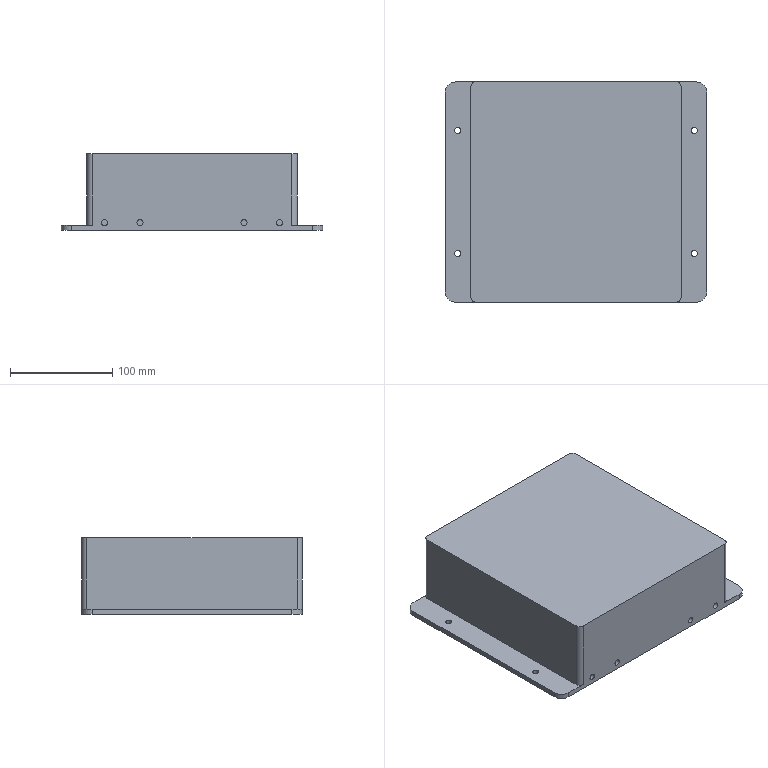NC program | NX | posted with a generic post | part box 255 x 215 x 75 mm
Lines 4678 to 5784 of 11258:
(ZLEVEL_PROFILE_COPY , TOOL : D10JING)
N9336 T14 M6
N9338 G54
N9340 G17 G0 G90 X87.615 Y-95.5 B0. C0. S9500 M3
N9342 G43 Z30. H14
N9344 Z0.5
N9346 G94 G1 Z-0.5 F1250.
N9348 X88.481 Y-97.
N9350 G3 X89.347 Y-97.5 R1.
N9352 G1 X92.492
N9354 X92.5 Y-97.459
N9356 Y-94.347
N9358 G3 X92. Y-93.481 R1.
N9360 G1 X90.5 Y-92.615
N9362 Z0.5
N9364 G0 X87.615 Y-95.5 Z0.
N9366 G1 Z-1.
N9368 X88.481 Y-97.
N9370 G3 X89.347 Y-97.5 R1.
N9372 G1 X92.492
N9374 X92.5 Y-97.459
N9376 Y-94.347
N9378 G3 X92. Y-93.481 R1.
N9380 G1 X90.5 Y-92.615
N9382 Z0.
N9384 G0 X87.615 Y-95.5 Z-0.5
N9386 G1 Z-1.5
N9388 X88.481 Y-97.
N9390 G3 X89.347 Y-97.5 R1.
N9392 G1 X92.492
N9394 X92.5 Y-97.459
N9396 Y-94.347
N9398 G3 X92. Y-93.481 R1.
N9400 G1 X90.5 Y-92.615
N9402 Z-0.5
N9404 G0 X87.615 Y-95.5 Z-1.
N9406 G1 Z-2.
N9408 X88.481 Y-97.
N9410 G3 X89.347 Y-97.5 R1.
N9412 G1 X92.492
N9414 X92.5 Y-97.459
N9416 Y-94.347
N9418 G3 X92. Y-93.481 R1.
N9420 G1 X90.5 Y-92.615
N9422 Z-1.
N9424 G0 X87.615 Y-95.5 Z-1.5
N9426 G1 Z-2.5
N9428 X88.481 Y-97.
N9430 G3 X89.347 Y-97.5 R1.
N9432 G1 X92.492
N9434 X92.5 Y-97.459
N9436 Y-94.347
N9438 G3 X92. Y-93.481 R1.
N9440 G1 X90.5 Y-92.615
N9442 Z-1.5
N9444 G0 X87.615 Y-95.5 Z-2.
N9446 G1 Z-3.
N9448 X88.481 Y-97.
N9450 G3 X89.347 Y-97.5 R1.
N9452 G1 X92.492
N9454 X92.5 Y-97.459
N9456 Y-94.347
N9458 G3 X92. Y-93.481 R1.
N9460 G1 X90.5 Y-92.615
N9462 Z-2.
N9464 G0 X87.615 Y-95.5 Z-2.5
N9466 G1 Z-3.5
N9468 X88.481 Y-97.
N9470 G3 X89.347 Y-97.5 R1.
N9472 G1 X92.492
N9474 X92.5 Y-97.459
N9476 Y-94.347
N9478 G3 X92. Y-93.481 R1.
N9480 G1 X90.5 Y-92.615
N9482 Z-2.5
N9484 G0 X87.615 Y-95.5 Z-3.
N9486 G1 Z-4.
N9488 X88.481 Y-97.
N9490 G3 X89.347 Y-97.5 R1.
N9492 G1 X92.492
N9494 X92.5 Y-97.459
N9496 Y-94.347
N9498 G3 X92. Y-93.481 R1.
N9500 G1 X90.5 Y-92.615
N9502 Z-3.
N9504 G0 X87.615 Y-95.5 Z-3.5
N9506 G1 Z-4.5
N9508 X88.481 Y-97.
N9510 G3 X89.347 Y-97.5 R1.
N9512 G1 X92.492
N9514 X92.5 Y-97.459
N9516 Y-94.347
N9518 G3 X92. Y-93.481 R1.
N9520 G1 X90.5 Y-92.615
N9522 Z-3.5
N9524 G0 X87.615 Y-95.5 Z-4.
N9526 G1 Z-5.
N9528 X88.481 Y-97.
N9530 G3 X89.347 Y-97.5 R1.
N9532 G1 X92.492
N9534 X92.5 Y-97.459
N9536 Y-94.347
N9538 G3 X92. Y-93.481 R1.
N9540 G1 X90.5 Y-92.615
N9542 Z-4.
N9544 G0 X87.615 Y-95.5 Z-4.5
N9546 G1 Z-5.5
N9548 X88.481 Y-97.
N9550 G3 X89.347 Y-97.5 R1.
N9552 G1 X92.492
N9554 X92.5 Y-97.459
N9556 Y-94.347
N9558 G3 X92. Y-93.481 R1.
N9560 G1 X90.5 Y-92.615
N9562 Z-4.5
N9564 G0 X87.615 Y-95.5 Z-5.
N9566 G1 Z-6.
N9568 X88.481 Y-97.
N9570 G3 X89.347 Y-97.5 R1.
N9572 G1 X92.492
N9574 X92.5 Y-97.459
N9576 Y-94.347
N9578 G3 X92. Y-93.481 R1.
N9580 G1 X90.5 Y-92.615
N9582 Z-5.
N9584 G0 X87.615 Y-95.5 Z-5.5
N9586 G1 Z-6.5
N9588 X88.481 Y-97.
N9590 G3 X89.347 Y-97.5 R1.
N9592 G1 X92.492
N9594 X92.5 Y-97.459
N9596 Y-94.347
N9598 G3 X92. Y-93.481 R1.
N9600 G1 X90.5 Y-92.615
N9602 Z-5.5
N9604 G0 X87.615 Y-95.5 Z-6.
N9606 G1 Z-7.
N9608 X88.481 Y-97.
N9610 G3 X89.347 Y-97.5 R1.
N9612 G1 X92.492
N9614 X92.5 Y-97.459
N9616 Y-94.347
N9618 G3 X92. Y-93.481 R1.
N9620 G1 X90.5 Y-92.615
N9622 Z-6.
N9624 G0 X87.615 Y-95.5 Z-6.5
N9626 G1 Z-7.5
N9628 X88.481 Y-97.
N9630 G3 X89.347 Y-97.5 R1.
N9632 G1 X92.492
N9634 X92.5 Y-97.459
N9636 Y-94.347
N9638 G3 X92. Y-93.481 R1.
N9640 G1 X90.5 Y-92.615
N9642 Z-6.5
N9644 G0 X87.615 Y-95.5 Z-7.
N9646 G1 Z-8.
N9648 X88.481 Y-97.
N9650 G3 X89.347 Y-97.5 R1.
N9652 G1 X92.492
N9654 X92.5 Y-97.459
N9656 Y-94.347
N9658 G3 X92. Y-93.481 R1.
N9660 G1 X90.5 Y-92.615
N9662 Z-7.
N9664 G0 X87.615 Y-95.5 Z-7.5
N9666 G1 Z-8.5
N9668 X88.481 Y-97.
N9670 G3 X89.347 Y-97.5 R1.
N9672 G1 X92.492
N9674 X92.5 Y-97.459
N9676 Y-94.347
N9678 G3 X92. Y-93.481 R1.
N9680 G1 X90.5 Y-92.615
N9682 Z-7.5
N9684 G0 X87.615 Y-95.5 Z-8.
N9686 G1 Z-9.
N9688 X88.481 Y-97.
N9690 G3 X89.347 Y-97.5 R1.
N9692 G1 X92.492
N9694 X92.5 Y-97.459
N9696 Y-94.347
N9698 G3 X92. Y-93.481 R1.
N9700 G1 X90.5 Y-92.615
N9702 Z-8.
N9704 G0 X87.615 Y-95.5 Z-8.5
N9706 G1 Z-9.5
N9708 X88.481 Y-97.
N9710 G3 X89.347 Y-97.5 R1.
N9712 G1 X92.492
N9714 X92.5 Y-97.459
N9716 Y-94.347
N9718 G3 X92. Y-93.481 R1.
N9720 G1 X90.5 Y-92.615
N9722 Z-8.5
N9724 G0 X87.615 Y-95.5 Z-9.
N9726 G1 Z-10.
N9728 X88.481 Y-97.
N9730 G3 X89.347 Y-97.5 R1.
N9732 G1 X92.492
N9734 X92.5 Y-97.459
N9736 Y-94.347
N9738 G3 X92. Y-93.481 R1.
N9740 G1 X90.5 Y-92.615
N9742 Z-9.
N9744 G0 X87.615 Y-95.5 Z-9.5
N9746 G1 Z-10.5
N9748 X88.481 Y-97.
N9750 G3 X89.347 Y-97.5 R1.
N9752 G1 X92.492
N9754 X92.5 Y-97.459
N9756 Y-94.347
N9758 G3 X92. Y-93.481 R1.
N9760 G1 X90.5 Y-92.615
N9762 Z-9.5
N9764 G0 X87.615 Y-95.5 Z-10.
N9766 G1 Z-11.
N9768 X88.481 Y-97.
N9770 G3 X89.347 Y-97.5 R1.
N9772 G1 X92.492
N9774 X92.5 Y-97.459
N9776 Y-94.347
N9778 G3 X92. Y-93.481 R1.
N9780 G1 X90.5 Y-92.615
N9782 Z-10.
N9784 G0 X87.615 Y-95.5 Z-10.5
N9786 G1 Z-11.5
N9788 X88.481 Y-97.
N9790 G3 X89.347 Y-97.5 R1.
N9792 G1 X92.492
N9794 X92.5 Y-97.459
N9796 Y-94.347
N9798 G3 X92. Y-93.481 R1.
N9800 G1 X90.5 Y-92.615
N9802 Z-10.5
N9804 G0 X87.615 Y-95.5 Z-11.
N9806 G1 Z-12.
N9808 X88.481 Y-97.
N9810 G3 X89.347 Y-97.5 R1.
N9812 G1 X92.492
N9814 X92.5 Y-97.459
N9816 Y-94.347
N9818 G3 X92. Y-93.481 R1.
N9820 G1 X90.5 Y-92.615
N9822 Z-11.
N9824 G0 X87.615 Y-95.5 Z-11.5
N9826 G1 Z-12.5
N9828 X88.481 Y-97.
N9830 G3 X89.347 Y-97.5 R1.
N9832 G1 X92.492
N9834 X92.5 Y-97.459
N9836 Y-94.347
N9838 G3 X92. Y-93.481 R1.
N9840 G1 X90.5 Y-92.615
N9842 Z-11.5
N9844 G0 X87.615 Y-95.5 Z-12.
N9846 G1 Z-13.
N9848 X88.481 Y-97.
N9850 G3 X89.347 Y-97.5 R1.
N9852 G1 X92.492
N9854 X92.5 Y-97.459
N9856 Y-94.347
N9858 G3 X92. Y-93.481 R1.
N9860 G1 X90.5 Y-92.615
N9862 Z-12.
N9864 G0 X87.615 Y-95.5 Z-12.5
N9866 G1 Z-13.5
N9868 X88.481 Y-97.
N9870 G3 X89.347 Y-97.5 R1.
N9872 G1 X92.492
N9874 X92.5 Y-97.459
N9876 Y-94.347
N9878 G3 X92. Y-93.481 R1.
N9880 G1 X90.5 Y-92.615
N9882 Z-12.5
N9884 G0 X87.615 Y-95.5 Z-13.
N9886 G1 Z-14.
N9888 X88.481 Y-97.
N9890 G3 X89.347 Y-97.5 R1.
N9892 G1 X92.492
N9894 X92.5 Y-97.459
N9896 Y-94.347
N9898 G3 X92. Y-93.481 R1.
N9900 G1 X90.5 Y-92.615
N9902 Z-13.
N9904 G0 X87.615 Y-95.5 Z-13.5
N9906 G1 Z-14.5
N9908 X88.481 Y-97.
N9910 G3 X89.347 Y-97.5 R1.
N9912 G1 X92.492
N9914 X92.5 Y-97.459
N9916 Y-94.347
N9918 G3 X92. Y-93.481 R1.
N9920 G1 X90.5 Y-92.615
N9922 Z-13.5
N9924 G0 X87.615 Y-95.5 Z-14.
N9926 G1 Z-15.
N9928 X88.481 Y-97.
N9930 G3 X89.347 Y-97.5 R1.
N9932 G1 X92.492
N9934 X92.5 Y-97.459
N9936 Y-94.347
N9938 G3 X92. Y-93.481 R1.
N9940 G1 X90.5 Y-92.615
N9942 Z-14.
N9944 G0 X87.615 Y-95.5 Z-14.5
N9946 G1 Z-15.5
N9948 X88.481 Y-97.
N9950 G3 X89.347 Y-97.5 R1.
N9952 G1 X92.492
N9954 X92.5 Y-97.459
N9956 Y-94.347
N9958 G3 X92. Y-93.481 R1.
N9960 G1 X90.5 Y-92.615
N9962 Z-14.5
N9964 G0 X87.615 Y-95.5 Z-15.
N9966 G1 Z-16.
N9968 X88.481 Y-97.
N9970 G3 X89.347 Y-97.5 R1.
N9972 G1 X92.492
N9974 X92.5 Y-97.459
N9976 Y-94.347
N9978 G3 X92. Y-93.481 R1.
N9980 G1 X90.5 Y-92.615
N9982 Z-15.
N9984 G0 X87.615 Y-95.5 Z-15.5
N9986 G1 Z-16.5
N9988 X88.481 Y-97.
N9990 G3 X89.347 Y-97.5 R1.
N9992 G1 X92.492
N9994 X92.5 Y-97.459
N9996 Y-94.347
N9998 G3 X92. Y-93.481 R1.
N10000 G1 X90.5 Y-92.615
N10002 Z-15.5
N10004 G0 X87.615 Y-95.5 Z-16.
N10006 G1 Z-17.
N10008 X88.481 Y-97.
N10010 G3 X89.347 Y-97.5 R1.
N10012 G1 X92.492
N10014 X92.5 Y-97.459
N10016 Y-94.347
N10018 G3 X92. Y-93.481 R1.
N10020 G1 X90.5 Y-92.615
N10022 Z-16.
N10024 G0 X87.615 Y-95.5 Z-16.5
N10026 G1 Z-17.5
N10028 X88.481 Y-97.
N10030 G3 X89.347 Y-97.5 R1.
N10032 G1 X92.492
N10034 X92.5 Y-97.459
N10036 Y-94.347
N10038 G3 X92. Y-93.481 R1.
N10040 G1 X90.5 Y-92.615
N10042 Z-16.5
N10044 G0 X87.615 Y-95.5 Z-17.
N10046 G1 Z-18.
N10048 X88.481 Y-97.
N10050 G3 X89.347 Y-97.5 R1.
N10052 G1 X92.492
N10054 X92.5 Y-97.459
N10056 Y-94.347
N10058 G3 X92. Y-93.481 R1.
N10060 G1 X90.5 Y-92.615
N10062 Z-17.
N10064 G0 X87.615 Y-95.5 Z-17.5
N10066 G1 Z-18.5
N10068 X88.481 Y-97.
N10070 G3 X89.347 Y-97.5 R1.
N10072 G1 X92.492
N10074 X92.5 Y-97.459
N10076 Y-94.347
N10078 G3 X92. Y-93.481 R1.
N10080 G1 X90.5 Y-92.615
N10082 Z-17.5
N10084 G0 X87.615 Y-95.5 Z-18.
N10086 G1 Z-19.
N10088 X88.481 Y-97.
N10090 G3 X89.347 Y-97.5 R1.
N10092 G1 X92.492
N10094 X92.5 Y-97.459
N10096 Y-94.347
N10098 G3 X92. Y-93.481 R1.
N10100 G1 X90.5 Y-92.615
N10102 Z-18.
N10104 G0 X87.615 Y-95.5 Z-18.5
N10106 G1 Z-19.5
N10108 X88.481 Y-97.
N10110 G3 X89.347 Y-97.5 R1.
N10112 G1 X92.492
N10114 X92.5 Y-97.459
N10116 Y-94.347
N10118 G3 X92. Y-93.481 R1.
N10120 G1 X90.5 Y-92.615
N10122 Z-18.5
N10124 G0 X87.615 Y-95.5 Z-19.
N10126 G1 Z-20.
N10128 X88.481 Y-97.
N10130 G3 X89.347 Y-97.5 R1.
N10132 G1 X92.492
N10134 X92.5 Y-97.459
N10136 Y-94.347
N10138 G3 X92. Y-93.481 R1.
N10140 G1 X90.5 Y-92.615
N10142 Z-19.
N10144 G0 X87.615 Y-95.5 Z-19.5
N10146 G1 Z-20.5
N10148 X88.481 Y-97.
N10150 G3 X89.347 Y-97.5 R1.
N10152 G1 X92.492
N10154 X92.5 Y-97.459
N10156 Y-94.347
N10158 G3 X92. Y-93.481 R1.
N10160 G1 X90.5 Y-92.615
N10162 Z-19.5
N10164 G0 X87.615 Y-95.5 Z-20.
N10166 G1 Z-21.
N10168 X88.481 Y-97.
N10170 G3 X89.347 Y-97.5 R1.
N10172 G1 X92.492
N10174 X92.5 Y-97.459
N10176 Y-94.347
N10178 G3 X92. Y-93.481 R1.
N10180 G1 X90.5 Y-92.615
N10182 Z-20.
N10184 G0 X87.615 Y-95.5 Z-20.5
N10186 G1 Z-21.5
N10188 X88.481 Y-97.
N10190 G3 X89.347 Y-97.5 R1.
N10192 G1 X92.492
N10194 X92.5 Y-97.459
N10196 Y-94.347
N10198 G3 X92. Y-93.481 R1.
N10200 G1 X90.5 Y-92.615
N10202 Z-20.5
N10204 G0 X87.615 Y-95.5 Z-21.
N10206 G1 Z-22.
N10208 X88.481 Y-97.
N10210 G3 X89.347 Y-97.5 R1.
N10212 G1 X92.492
N10214 X92.5 Y-97.459
N10216 Y-94.347
N10218 G3 X92. Y-93.481 R1.
N10220 G1 X90.5 Y-92.615
N10222 Z-21.
N10224 G0 X87.615 Y-95.5 Z-21.5
N10226 G1 Z-22.5
N10228 X88.481 Y-97.
N10230 G3 X89.347 Y-97.5 R1.
N10232 G1 X92.492
N10234 X92.5 Y-97.459
N10236 Y-94.347
N10238 G3 X92. Y-93.481 R1.
N10240 G1 X90.5 Y-92.615
N10242 Z-21.5
N10244 G0 X87.615 Y-95.5 Z-22.
N10246 G1 Z-23.
N10248 X88.481 Y-97.
N10250 G3 X89.347 Y-97.5 R1.
N10252 G1 X92.492
N10254 X92.5 Y-97.459
N10256 Y-94.347
N10258 G3 X92. Y-93.481 R1.
N10260 G1 X90.5 Y-92.615
N10262 Z-22.
N10264 G0 X87.615 Y-95.5 Z-22.5
N10266 G1 Z-23.5
N10268 X88.481 Y-97.
N10270 G3 X89.347 Y-97.5 R1.
N10272 G1 X92.492
N10274 X92.5 Y-97.459
N10276 Y-94.347
N10278 G3 X92. Y-93.481 R1.
N10280 G1 X90.5 Y-92.615
N10282 Z-22.5
N10284 G0 X87.615 Y-95.5 Z-23.
N10286 G1 Z-24.
N10288 X88.481 Y-97.
N10290 G3 X89.347 Y-97.5 R1.
N10292 G1 X92.492
N10294 X92.5 Y-97.459
N10296 Y-94.347
N10298 G3 X92. Y-93.481 R1.
N10300 G1 X90.5 Y-92.615
N10302 Z-23.
N10304 G0 X87.615 Y-95.5 Z-23.5
N10306 G1 Z-24.5
N10308 X88.481 Y-97.
N10310 G3 X89.347 Y-97.5 R1.
N10312 G1 X92.492
N10314 X92.5 Y-97.459
N10316 Y-94.347
N10318 G3 X92. Y-93.481 R1.
N10320 G1 X90.5 Y-92.615
N10322 Z-23.5
N10324 G0 X87.615 Y-95.5 Z-24.
N10326 G1 Z-25.
N10328 X88.481 Y-97.
N10330 G3 X89.347 Y-97.5 R1.
N10332 G1 X92.492
N10334 X92.5 Y-97.459
N10336 Y-94.347
N10338 G3 X92. Y-93.481 R1.
N10340 G1 X90.5 Y-92.615
N10342 Z-24.
N10344 G0 X87.615 Y-95.5 Z-24.5
N10346 G1 Z-25.5
N10348 X88.481 Y-97.
N10350 G3 X89.347 Y-97.5 R1.
N10352 G1 X92.492
N10354 X92.5 Y-97.459
N10356 Y-94.347
N10358 G3 X92. Y-93.481 R1.
N10360 G1 X90.5 Y-92.615
N10362 Z-24.5
N10364 G0 X87.615 Y-95.5 Z-25.
N10366 G1 Z-26.
N10368 X88.481 Y-97.
N10370 G3 X89.347 Y-97.5 R1.
N10372 G1 X92.492
N10374 X92.5 Y-97.459
N10376 Y-94.347
N10378 G3 X92. Y-93.481 R1.
N10380 G1 X90.5 Y-92.615
N10382 Z-25.
N10384 G0 X87.615 Y-95.5 Z-25.5
N10386 G1 Z-26.5
N10388 X88.481 Y-97.
N10390 G3 X89.347 Y-97.5 R1.
N10392 G1 X92.492
N10394 X92.5 Y-97.459
N10396 Y-94.347
N10398 G3 X92. Y-93.481 R1.
N10400 G1 X90.5 Y-92.615
N10402 Z-25.5
N10404 G0 X87.615 Y-95.5 Z-26.
N10406 G1 Z-27.
N10408 X88.481 Y-97.
N10410 G3 X89.347 Y-97.5 R1.
N10412 G1 X92.492
N10414 X92.5 Y-97.459
N10416 Y-94.347
N10418 G3 X92. Y-93.481 R1.
N10420 G1 X90.5 Y-92.615
N10422 Z-26.
N10424 G0 X87.615 Y-95.5 Z-26.5
N10426 G1 Z-27.5
N10428 X88.481 Y-97.
N10430 G3 X89.347 Y-97.5 R1.
N10432 G1 X92.492
N10434 X92.5 Y-97.459
N10436 Y-94.347
N10438 G3 X92. Y-93.481 R1.
N10440 G1 X90.5 Y-92.615
N10442 Z-26.5
N10444 G0 X87.615 Y-95.5 Z-27.
N10446 G1 Z-28.
N10448 X88.481 Y-97.
N10450 G3 X89.347 Y-97.5 R1.
N10452 G1 X92.492
N10454 X92.5 Y-97.459
N10456 Y-94.347
N10458 G3 X92. Y-93.481 R1.
N10460 G1 X90.5 Y-92.615
N10462 Z-27.
N10464 G0 X87.615 Y-95.5 Z-27.5
N10466 G1 Z-28.5
N10468 X88.481 Y-97.
N10470 G3 X89.347 Y-97.5 R1.
N10472 G1 X92.492
N10474 X92.5 Y-97.459
N10476 Y-94.347
N10478 G3 X92. Y-93.481 R1.
N10480 G1 X90.5 Y-92.615
N10482 Z-27.5
N10484 G0 X87.615 Y-95.5 Z-28.
N10486 G1 Z-29.
N10488 X88.481 Y-97.
N10490 G3 X89.347 Y-97.5 R1.
N10492 G1 X92.492
N10494 X92.5 Y-97.459
N10496 Y-94.347
N10498 G3 X92. Y-93.481 R1.
N10500 G1 X90.5 Y-92.615
N10502 Z-28.
N10504 G0 X87.615 Y-95.5 Z-28.5
N10506 G1 Z-29.5
N10508 X88.481 Y-97.
N10510 G3 X89.347 Y-97.5 R1.
N10512 G1 X92.492
N10514 X92.5 Y-97.459
N10516 Y-94.347
N10518 G3 X92. Y-93.481 R1.
N10520 G1 X90.5 Y-92.615
N10522 Z-28.5
N10524 G0 X87.615 Y-95.5 Z-29.
N10526 G1 Z-30.
N10528 X88.481 Y-97.
N10530 G3 X89.347 Y-97.5 R1.
N10532 G1 X92.492
N10534 X92.5 Y-97.459
N10536 Y-94.347
N10538 G3 X92. Y-93.481 R1.
N10540 G1 X90.5 Y-92.615
N10542 Z-29.
N10544 G0 X87.615 Y-95.5 Z-29.5
N10546 G1 Z-30.5
N10548 X88.481 Y-97.
N10550 G3 X89.347 Y-97.5 R1.
N10552 G1 X92.492
N10554 X92.5 Y-97.459
N10556 Y-94.347
N10558 G3 X92. Y-93.481 R1.
N10560 G1 X90.5 Y-92.615
N10562 Z-29.5
N10564 G0 X87.615 Y-95.5 Z-30.
N10566 G1 Z-31.
N10568 X88.481 Y-97.
N10570 G3 X89.347 Y-97.5 R1.
N10572 G1 X92.492
N10574 X92.5 Y-97.459
N10576 Y-94.347
N10578 G3 X92. Y-93.481 R1.
N10580 G1 X90.5 Y-92.615
N10582 Z-30.
N10584 G0 X87.615 Y-95.5 Z-30.5
N10586 G1 Z-31.5
N10588 X88.481 Y-97.
N10590 G3 X89.347 Y-97.5 R1.
N10592 G1 X92.492
N10594 X92.5 Y-97.459
N10596 Y-94.347
N10598 G3 X92. Y-93.481 R1.
N10600 G1 X90.5 Y-92.615
N10602 Z-30.5
N10604 G0 X87.615 Y-95.5 Z-31.
N10606 G1 Z-32.
N10608 X88.481 Y-97.
N10610 G3 X89.347 Y-97.5 R1.
N10612 G1 X92.492
N10614 X92.5 Y-97.459
N10616 Y-94.347
N10618 G3 X92. Y-93.481 R1.
N10620 G1 X90.5 Y-92.615
N10622 Z-31.
N10624 G0 X87.615 Y-95.5 Z-31.5
N10626 G1 Z-32.5
N10628 X88.481 Y-97.
N10630 G3 X89.347 Y-97.5 R1.
N10632 G1 X92.492
N10634 X92.5 Y-97.459
N10636 Y-94.347
N10638 G3 X92. Y-93.481 R1.
N10640 G1 X90.5 Y-92.615
N10642 Z-31.5
N10644 G0 X87.615 Y-95.5 Z-32.
N10646 G1 Z-33.
N10648 X88.481 Y-97.
N10650 G3 X89.347 Y-97.5 R1.
N10652 G1 X92.492
N10654 X92.5 Y-97.459
N10656 Y-94.347
N10658 G3 X92. Y-93.481 R1.
N10660 G1 X90.5 Y-92.615
N10662 Z-32.
N10664 G0 X87.615 Y-95.5 Z-32.5
N10666 G1 Z-33.5
N10668 X88.481 Y-97.
N10670 G3 X89.347 Y-97.5 R1.
N10672 G1 X92.492
N10674 X92.5 Y-97.459
N10676 Y-94.347
N10678 G3 X92. Y-93.481 R1.
N10680 G1 X90.5 Y-92.615
N10682 Z-32.5
N10684 G0 X87.615 Y-95.5 Z-33.
N10686 G1 Z-34.
N10688 X88.481 Y-97.
N10690 G3 X89.347 Y-97.5 R1.
N10692 G1 X92.492
N10694 X92.5 Y-97.459
N10696 Y-94.347
N10698 G3 X92. Y-93.481 R1.
N10700 G1 X90.5 Y-92.615
N10702 Z-33.
N10704 G0 X87.615 Y-95.5 Z-33.5
N10706 G1 Z-34.5
N10708 X88.481 Y-97.
N10710 G3 X89.347 Y-97.5 R1.
N10712 G1 X92.492
N10714 X92.5 Y-97.459
N10716 Y-94.347
N10718 G3 X92. Y-93.481 R1.
N10720 G1 X90.5 Y-92.615
N10722 Z-33.5
N10724 G0 X87.615 Y-95.5 Z-34.
N10726 G1 Z-35.
N10728 X88.481 Y-97.
N10730 G3 X89.347 Y-97.5 R1.
N10732 G1 X92.492
N10734 X92.5 Y-97.459
N10736 Y-94.347
N10738 G3 X92. Y-93.481 R1.
N10740 G1 X90.5 Y-92.615
N10742 Z-34.
N10744 G0 X87.615 Y-95.5 Z-34.5
N10746 G1 Z-35.5
N10748 X88.481 Y-97.
N10750 G3 X89.347 Y-97.5 R1.
N10752 G1 X92.492
N10754 X92.5 Y-97.459
N10756 Y-94.347
N10758 G3 X92. Y-93.481 R1.
N10760 G1 X90.5 Y-92.615
N10762 Z-34.5
N10764 G0 X87.615 Y-95.5 Z-35.
N10766 G1 Z-36.
N10768 X88.481 Y-97.
N10770 G3 X89.347 Y-97.5 R1.
N10772 G1 X92.492
N10774 X92.5 Y-97.459
N10776 Y-94.347
N10778 G3 X92. Y-93.481 R1.
N10780 G1 X90.5 Y-92.615
N10782 Z-35.
N10784 G0 X87.615 Y-95.5 Z-35.5
N10786 G1 Z-36.5
N10788 X88.481 Y-97.
N10790 G3 X89.347 Y-97.5 R1.
N10792 G1 X92.492
N10794 X92.5 Y-97.459
N10796 Y-94.347
N10798 G3 X92. Y-93.481 R1.
N10800 G1 X90.5 Y-92.615
N10802 Z-35.5
N10804 G0 X87.615 Y-95.5 Z-36.
N10806 G1 Z-37.
N10808 X88.481 Y-97.
N10810 G3 X89.347 Y-97.5 R1.
N10812 G1 X92.492
N10814 X92.5 Y-97.459
N10816 Y-94.347
N10818 G3 X92. Y-93.481 R1.
N10820 G1 X90.5 Y-92.615
N10822 Z-36.
N10824 G0 X87.615 Y-95.5 Z-36.5
N10826 G1 Z-37.5
N10828 X88.481 Y-97.
N10830 G3 X89.347 Y-97.5 R1.
N10832 G1 X92.492
N10834 X92.5 Y-97.459
N10836 Y-94.347
N10838 G3 X92. Y-93.481 R1.
N10840 G1 X90.5 Y-92.615
N10842 Z-36.5
N10844 G0 X87.615 Y-95.5 Z-37.
N10846 G1 Z-38.
N10848 X88.481 Y-97.
N10850 G3 X89.347 Y-97.5 R1.
N10852 G1 X92.492
N10854 X92.5 Y-97.459
N10856 Y-94.347
N10858 G3 X92. Y-93.481 R1.
N10860 G1 X90.5 Y-92.615
N10862 Z-37.
N10864 G0 X87.615 Y-95.5 Z-37.5
N10866 G1 Z-38.5
N10868 X88.481 Y-97.
N10870 G3 X89.347 Y-97.5 R1.
N10872 G1 X92.492
N10874 X92.5 Y-97.459
N10876 Y-94.347
N10878 G3 X92. Y-93.481 R1.
N10880 G1 X90.5 Y-92.615
N10882 Z-37.5
N10884 G0 X87.615 Y-95.5 Z-38.
N10886 G1 Z-39.
N10888 X88.481 Y-97.
N10890 G3 X89.347 Y-97.5 R1.
N10892 G1 X92.492
N10894 X92.5 Y-97.459
N10896 Y-94.347
N10898 G3 X92. Y-93.481 R1.
N10900 G1 X90.5 Y-92.615
N10902 Z-38.
N10904 G0 X87.615 Y-95.5 Z-38.5
N10906 G1 Z-39.5
N10908 X88.481 Y-97.
N10910 G3 X89.347 Y-97.5 R1.
N10912 G1 X92.492
N10914 X92.5 Y-97.459
N10916 Y-94.347
N10918 G3 X92. Y-93.481 R1.
N10920 G1 X90.5 Y-92.615
N10922 Z-38.5
N10924 G0 X87.615 Y-95.5 Z-39.
N10926 G1 Z-40.
N10928 X88.481 Y-97.
N10930 G3 X89.347 Y-97.5 R1.
N10932 G1 X92.492
N10934 X92.5 Y-97.459
N10936 Y-94.347
N10938 G3 X92. Y-93.481 R1.
N10940 G1 X90.5 Y-92.615
N10942 Z-39.
N10944 G0 X87.615 Y-95.5 Z-39.5
N10946 G1 Z-40.5
N10948 X88.481 Y-97.
N10950 G3 X89.347 Y-97.5 R1.
N10952 G1 X92.492
N10954 X92.5 Y-97.459
N10956 Y-94.347
N10958 G3 X92. Y-93.481 R1.
N10960 G1 X90.5 Y-92.615
N10962 Z-39.5
N10964 G0 X87.615 Y-95.5 Z-40.
N10966 G1 Z-41.
N10968 X88.481 Y-97.
N10970 G3 X89.347 Y-97.5 R1.
N10972 G1 X92.492
N10974 X92.5 Y-97.459
N10976 Y-94.347
N10978 G3 X92. Y-93.481 R1.
N10980 G1 X90.5 Y-92.615
N10982 Z-40.
N10984 G0 X87.615 Y-95.5 Z-40.5
N10986 G1 Z-41.5
N10988 X88.481 Y-97.
N10990 G3 X89.347 Y-97.5 R1.
N10992 G1 X92.492
N10994 X92.5 Y-97.459
N10996 Y-94.347
N10998 G3 X92. Y-93.481 R1.
N11000 G1 X90.5 Y-92.615
N11002 Z-40.5
N11004 G0 X87.615 Y-95.5 Z-41.
N11006 G1 Z-42.
N11008 X88.481 Y-97.
N11010 G3 X89.347 Y-97.5 R1.
N11012 G1 X92.492
N11014 X92.5 Y-97.459
N11016 Y-94.347
N11018 G3 X92. Y-93.481 R1.
N11020 G1 X90.5 Y-92.615
N11022 Z-41.
N11024 G0 X87.615 Y-95.5 Z-41.5
N11026 G1 Z-42.5
N11028 X88.481 Y-97.
N11030 G3 X89.347 Y-97.5 R1.
N11032 G1 X92.492
N11034 X92.5 Y-97.459
N11036 Y-94.347
N11038 G3 X92. Y-93.481 R1.
N11040 G1 X90.5 Y-92.615
N11042 Z-41.5
N11044 G0 X87.615 Y-95.5 Z-42.
N11046 G1 Z-43.
N11048 X88.481 Y-97.
N11050 G3 X89.347 Y-97.5 R1.
N11052 G1 X92.492
N11054 X92.5 Y-97.459
N11056 Y-94.347
N11058 G3 X92. Y-93.481 R1.
N11060 G1 X90.5 Y-92.615
N11062 Z-42.
N11064 G0 X87.615 Y-95.5 Z-42.5
N11066 G1 Z-43.5
N11068 X88.481 Y-97.
N11070 G3 X89.347 Y-97.5 R1.
N11072 G1 X92.492
N11074 X92.5 Y-97.459
N11076 Y-94.347
N11078 G3 X92. Y-93.481 R1.
N11080 G1 X90.5 Y-92.615
N11082 Z-42.5
N11084 G0 X87.615 Y-95.5 Z-43.
N11086 G1 Z-44.
N11088 X88.481 Y-97.
N11090 G3 X89.347 Y-97.5 R1.
N11092 G1 X92.492
N11094 X92.5 Y-97.459
N11096 Y-94.347
N11098 G3 X92. Y-93.481 R1.
N11100 G1 X90.5 Y-92.615
N11102 Z-43.
N11104 G0 X87.615 Y-95.5 Z-43.5
N11106 G1 Z-44.5
N11108 X88.481 Y-97.
N11110 G3 X89.347 Y-97.5 R1.
N11112 G1 X92.492
N11114 X92.5 Y-97.459
N11116 Y-94.347
N11118 G3 X92. Y-93.481 R1.
N11120 G1 X90.5 Y-92.615
N11122 Z-43.5
N11124 G0 X87.615 Y-95.5 Z-44.
N11126 G1 Z-45.
N11128 X88.481 Y-97.
N11130 G3 X89.347 Y-97.5 R1.
N11132 G1 X92.492
N11134 X92.5 Y-97.459
N11136 Y-94.347
N11138 G3 X92. Y-93.481 R1.
N11140 G1 X90.5 Y-92.615
N11142 Z-44.
N11144 G0 X87.615 Y-95.5 Z-44.5
N11146 G1 Z-45.5
N11148 X88.481 Y-97.
N11150 G3 X89.347 Y-97.5 R1.
N11152 G1 X92.492
N11154 X92.5 Y-97.459
N11156 Y-94.347
N11158 G3 X92. Y-93.481 R1.
N11160 G1 X90.5 Y-92.615
N11162 Z-44.5
N11164 G0 X87.615 Y-95.5 Z-45.
N11166 G1 Z-46.
N11168 X88.481 Y-97.
N11170 G3 X89.347 Y-97.5 R1.
N11172 G1 X92.492
N11174 X92.5 Y-97.459
N11176 Y-94.347
N11178 G3 X92. Y-93.481 R1.
N11180 G1 X90.5 Y-92.615
N11182 Z-45.
N11184 G0 X87.615 Y-95.5 Z-45.5
N11186 G1 Z-46.5
N11188 X88.481 Y-97.
N11190 G3 X89.347 Y-97.5 R1.
N11192 G1 X92.492
N11194 X92.5 Y-97.459
N11196 Y-94.347
N11198 G3 X92. Y-93.481 R1.
N11200 G1 X90.5 Y-92.615
N11202 Z-45.5
N11204 G0 X87.615 Y-95.5 Z-46.
N11206 G1 Z-47.
N11208 X88.481 Y-97.
N11210 G3 X89.347 Y-97.5 R1.
N11212 G1 X92.492
N11214 X92.5 Y-97.459
N11216 Y-94.347
N11218 G3 X92. Y-93.481 R1.
N11220 G1 X90.5 Y-92.615
N11222 Z-46.
N11224 G0 X87.615 Y-95.5 Z-46.5
N11226 G1 Z-47.5
N11228 X88.481 Y-97.
N11230 G3 X89.347 Y-97.5 R1.
N11232 G1 X92.492
N11234 X92.5 Y-97.459
N11236 Y-94.347
N11238 G3 X92. Y-93.481 R1.
N11240 G1 X90.5 Y-92.615
N11242 Z-46.5
N11244 G0 X87.615 Y-95.5 Z-47.
N11246 G1 Z-48.
N11248 X88.481 Y-97.
N11250 G3 X89.347 Y-97.5 R1.
N11252 G1 X92.492
N11254 X92.5 Y-97.459
N11256 Y-94.347
N11258 G3 X92. Y-93.481 R1.
N11260 G1 X90.5 Y-92.615
N11262 Z-47.
N11264 G0 X87.615 Y-95.5 Z-47.5
N11266 G1 Z-48.5
N11268 X88.481 Y-97.
N11270 G3 X89.347 Y-97.5 R1.
N11272 G1 X92.492
N11274 X92.5 Y-97.459
N11276 Y-94.347
N11278 G3 X92. Y-93.481 R1.
N11280 G1 X90.5 Y-92.615
N11282 Z-47.5
N11284 G0 X87.615 Y-95.5 Z-48.
N11286 G1 Z-49.
N11288 X88.481 Y-97.
N11290 G3 X89.347 Y-97.5 R1.
N11292 G1 X92.492
N11294 X92.5 Y-97.459
N11296 Y-94.347
N11298 G3 X92. Y-93.481 R1.
N11300 G1 X90.5 Y-92.615
N11302 Z-48.
N11304 G0 X87.615 Y-95.5 Z-48.5
N11306 G1 Z-49.5
N11308 X88.481 Y-97.
N11310 G3 X89.347 Y-97.5 R1.
N11312 G1 X92.492
N11314 X92.5 Y-97.459
N11316 Y-94.347
N11318 G3 X92. Y-93.481 R1.
N11320 G1 X90.5 Y-92.615
N11322 Z-48.5
N11324 G0 X87.615 Y-95.5 Z-49.
N11326 G1 Z-50.
N11328 X88.481 Y-97.
N11330 G3 X89.347 Y-97.5 R1.
N11332 G1 X92.492
N11334 X92.5 Y-97.459
N11336 Y-94.347
N11338 G3 X92. Y-93.481 R1.
N11340 G1 X90.5 Y-92.615
N11342 Z-49.
N11344 G0 X87.615 Y-95.5 Z-49.5
N11346 G1 Z-50.5
N11348 X88.481 Y-97.
N11350 G3 X89.347 Y-97.5 R1.
N11352 G1 X92.492
N11354 X92.5 Y-97.459
N11356 Y-94.347
N11358 G3 X92. Y-93.481 R1.
N11360 G1 X90.5 Y-92.615
N11362 Z-49.5
N11364 G0 X87.615 Y-95.5 Z-50.
N11366 G1 Z-51.
N11368 X88.481 Y-97.
N11370 G3 X89.347 Y-97.5 R1.
N11372 G1 X92.492
N11374 X92.5 Y-97.459
N11376 Y-94.347
N11378 G3 X92. Y-93.481 R1.
N11380 G1 X90.5 Y-92.615
N11382 Z-50.
N11384 G0 X87.615 Y-95.5 Z-50.5
N11386 G1 Z-51.5
N11388 X88.481 Y-97.
N11390 G3 X89.347 Y-97.5 R1.
N11392 G1 X92.492
N11394 X92.5 Y-97.459
N11396 Y-94.347
N11398 G3 X92. Y-93.481 R1.
N11400 G1 X90.5 Y-92.615
N11402 Z-50.5
N11404 G0 X87.615 Y-95.5 Z-51.
N11406 G1 Z-52.
N11408 X88.481 Y-97.
N11410 G3 X89.347 Y-97.5 R1.
N11412 G1 X92.492
N11414 X92.5 Y-97.459
N11416 Y-94.347
N11418 G3 X92. Y-93.481 R1.
N11420 G1 X90.5 Y-92.615
N11422 Z-51.
N11424 G0 X87.615 Y-95.5 Z-51.5
N11426 G1 Z-52.5
N11428 X88.481 Y-97.
N11430 G3 X89.347 Y-97.5 R1.
N11432 G1 X92.492
N11434 X92.5 Y-97.459
N11436 Y-94.347
N11438 G3 X92. Y-93.481 R1.
N11440 G1 X90.5 Y-92.615
N11442 Z-51.5
N11444 G0 X87.615 Y-95.5 Z-52.
N11446 G1 Z-53.
N11448 X88.481 Y-97.
N11450 G3 X89.347 Y-97.5 R1.
N11452 G1 X92.492
N11454 X92.5 Y-97.459
N11456 Y-94.347
N11458 G3 X92. Y-93.481 R1.
N11460 G1 X90.5 Y-92.615
N11462 Z-52.
N11464 G0 X87.615 Y-95.5 Z-52.5
N11466 G1 Z-53.5
N11468 X88.481 Y-97.
N11470 G3 X89.347 Y-97.5 R1.
N11472 G1 X92.492
N11474 X92.5 Y-97.459
N11476 Y-94.347
N11478 G3 X92. Y-93.481 R1.
N11480 G1 X90.5 Y-92.615
N11482 Z-52.5
N11484 G0 X87.615 Y-95.5 Z-53.
N11486 G1 Z-54.
N11488 X88.481 Y-97.
N11490 G3 X89.347 Y-97.5 R1.
N11492 G1 X92.492
N11494 X92.5 Y-97.459
N11496 Y-94.347
N11498 G3 X92. Y-93.481 R1.
N11500 G1 X90.5 Y-92.615
N11502 Z-53.
N11504 G0 X87.615 Y-95.5 Z-53.5
N11506 G1 Z-54.5
N11508 X88.481 Y-97.
N11510 G3 X89.347 Y-97.5 R1.
N11512 G1 X92.492
N11514 X92.5 Y-97.459
N11516 Y-94.347
N11518 G3 X92. Y-93.481 R1.
N11520 G1 X90.5 Y-92.615
N11522 Z-53.5
N11524 G0 X87.615 Y-95.5 Z-54.
N11526 G1 Z-55.
N11528 X88.481 Y-97.
N11530 G3 X89.347 Y-97.5 R1.
N11532 G1 X92.492
N11534 X92.5 Y-97.459
N11536 Y-94.347
N11538 G3 X92. Y-93.481 R1.
N11540 G1 X90.5 Y-92.615
N11542 Z-54.